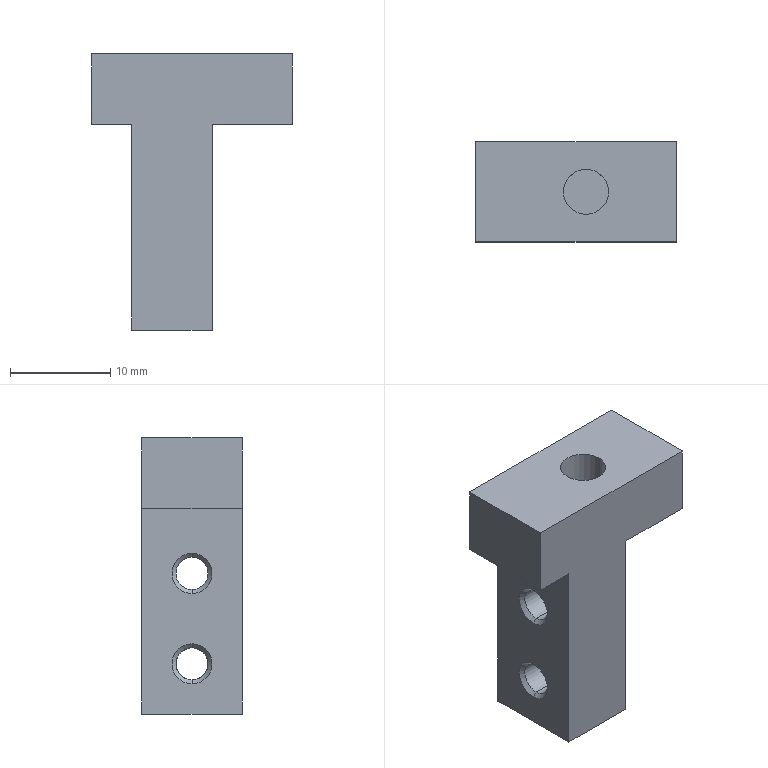Part | SolidWorks | features BaseBody 1 | 1 solid | 25 faces | box 20 x 10 x 27.5 mm | volume 2836 mm3 | plane 11 | cone 8 | cylinder 6 | commonest cylinder face diameters 3.2 x4 4.5 x2
STEP:
#1=CARTESIAN_POINT('',(-16.5,0.,-9.));
#2=VERTEX_POINT('',#1);
#3=CARTESIAN_POINT('',(-12.,0.,-9.));
#4=VERTEX_POINT('',#3);
#5=CARTESIAN_POINT('',(-14.25,0.,-9.));
#6=DIRECTION('',(0.,0.,1.));
#7=DIRECTION('',(1.,0.,0.));
#8=AXIS2_PLACEMENT_3D('',#5,#6,#7);
#9=CIRCLE('',#8,2.25);
#10=EDGE_CURVE('',#2,#4,#9,.T.);
#11=ORIENTED_EDGE('',*,*,#10,.F.);
#12=CARTESIAN_POINT('',(-16.5,0.,-4.5));
#13=VERTEX_POINT('',#12);
#14=CARTESIAN_POINT('',(-16.5,0.,-4.5));
#15=DIRECTION('',(0.,0.,1.));
#16=VECTOR('',#15,1000.);
#17=LINE('',#14,#16);
#18=EDGE_CURVE('',#2,#13,#17,.T.);
#19=ORIENTED_EDGE('',*,*,#18,.T.);
#20=CARTESIAN_POINT('',(-12.,0.,-4.5));
#21=VERTEX_POINT('',#20);
#22=CARTESIAN_POINT('',(-14.25,0.,-4.5));
#23=DIRECTION('',(0.,0.,-1.));
#24=DIRECTION('',(1.,0.,0.));
#25=AXIS2_PLACEMENT_3D('',#22,#23,#24);
#26=CIRCLE('',#25,2.25);
#27=EDGE_CURVE('',#21,#13,#26,.T.);
#28=ORIENTED_EDGE('',*,*,#27,.F.);
#29=CARTESIAN_POINT('',(-12.,0.,-4.5));
#30=DIRECTION('',(0.,0.,1.));
#31=VECTOR('',#30,1000.);
#32=LINE('',#29,#31);
#33=EDGE_CURVE('',#4,#21,#32,.T.);
#34=ORIENTED_EDGE('',*,*,#33,.F.);
#35=EDGE_LOOP('',(#11,#19,#28,#34));
#36=FACE_OUTER_BOUND('',#35,.T.);
#37=CARTESIAN_POINT('',(-14.25,0.,-4.5));
#38=DIRECTION('',(0.,0.,1.));
#39=DIRECTION('',(1.,0.,0.));
#40=AXIS2_PLACEMENT_3D('',#37,#38,#39);
#41=CYLINDRICAL_SURFACE('',#40,2.25);
#42=ADVANCED_FACE('',(#36),#41,.F.);
#43=CARTESIAN_POINT('',(-20.85,0.,-28.6));
#44=VERTEX_POINT('',#43);
#45=CARTESIAN_POINT('',(-20.85,0.,-25.4));
#46=VERTEX_POINT('',#45);
#47=CARTESIAN_POINT('',(-20.85,0.,-27.));
#48=DIRECTION('',(-1.,0.,0.));
#49=DIRECTION('',(0.,0.,-1.));
#50=AXIS2_PLACEMENT_3D('',#47,#48,#49);
#51=CIRCLE('',#50,1.6);
#52=EDGE_CURVE('',#44,#46,#51,.T.);
#53=ORIENTED_EDGE('',*,*,#52,.F.);
#54=CARTESIAN_POINT('',(-21.25,0.,-29.));
#55=VERTEX_POINT('',#54);
#56=CARTESIAN_POINT('',(-21.25,0.,-29.));
#57=DIRECTION('',(-0.7071,0.,-0.7071));
#58=VECTOR('',#57,1000.);
#59=LINE('',#56,#58);
#60=EDGE_CURVE('',#44,#55,#59,.T.);
#61=ORIENTED_EDGE('',*,*,#60,.T.);
#62=CARTESIAN_POINT('',(-21.25,0.,-25.));
#63=VERTEX_POINT('',#62);
#64=CARTESIAN_POINT('',(-21.25,0.,-27.));
#65=DIRECTION('',(1.,0.,0.));
#66=DIRECTION('',(0.,0.,1.));
#67=AXIS2_PLACEMENT_3D('',#64,#65,#66);
#68=CIRCLE('',#67,2.);
#69=EDGE_CURVE('',#63,#55,#68,.T.);
#70=ORIENTED_EDGE('',*,*,#69,.F.);
#71=CARTESIAN_POINT('',(-21.25,0.,-25.));
#72=DIRECTION('',(-0.7071,0.,0.7071));
#73=VECTOR('',#72,1000.);
#74=LINE('',#71,#73);
#75=EDGE_CURVE('',#46,#63,#74,.T.);
#76=ORIENTED_EDGE('',*,*,#75,.F.);
#77=EDGE_LOOP('',(#53,#61,#70,#76));
#78=FACE_OUTER_BOUND('',#77,.T.);
#79=CARTESIAN_POINT('',(-21.25,0.,-27.));
#80=DIRECTION('',(-1.,0.,0.));
#81=DIRECTION('',(0.,0.,1.));
#82=AXIS2_PLACEMENT_3D('',#79,#80,#81);
#83=CONICAL_SURFACE('',#82,2.,0.7854);
#84=ADVANCED_FACE('',(#78),#83,.F.);
#85=CARTESIAN_POINT('',(-20.85,0.,-19.6));
#86=VERTEX_POINT('',#85);
#87=CARTESIAN_POINT('',(-20.85,0.,-16.4));
#88=VERTEX_POINT('',#87);
#89=CARTESIAN_POINT('',(-20.85,0.,-18.));
#90=DIRECTION('',(-1.,0.,0.));
#91=DIRECTION('',(0.,0.,-1.));
#92=AXIS2_PLACEMENT_3D('',#89,#90,#91);
#93=CIRCLE('',#92,1.6);
#94=EDGE_CURVE('',#86,#88,#93,.T.);
#95=ORIENTED_EDGE('',*,*,#94,.F.);
#96=CARTESIAN_POINT('',(-21.25,0.,-20.));
#97=VERTEX_POINT('',#96);
#98=CARTESIAN_POINT('',(-21.25,0.,-20.));
#99=DIRECTION('',(-0.7071,0.,-0.7071));
#100=VECTOR('',#99,1000.);
#101=LINE('',#98,#100);
#102=EDGE_CURVE('',#86,#97,#101,.T.);
#103=ORIENTED_EDGE('',*,*,#102,.T.);
#104=CARTESIAN_POINT('',(-21.25,0.,-16.));
#105=VERTEX_POINT('',#104);
#106=CARTESIAN_POINT('',(-21.25,0.,-18.));
#107=DIRECTION('',(1.,0.,0.));
#108=DIRECTION('',(0.,0.,1.));
#109=AXIS2_PLACEMENT_3D('',#106,#107,#108);
#110=CIRCLE('',#109,2.);
#111=EDGE_CURVE('',#105,#97,#110,.T.);
#112=ORIENTED_EDGE('',*,*,#111,.F.);
#113=CARTESIAN_POINT('',(-21.25,0.,-16.));
#114=DIRECTION('',(-0.7071,0.,0.7071));
#115=VECTOR('',#114,1000.);
#116=LINE('',#113,#115);
#117=EDGE_CURVE('',#88,#105,#116,.T.);
#118=ORIENTED_EDGE('',*,*,#117,.F.);
#119=EDGE_LOOP('',(#95,#103,#112,#118));
#120=FACE_OUTER_BOUND('',#119,.T.);
#121=CARTESIAN_POINT('',(-21.25,0.,-18.));
#122=DIRECTION('',(-1.,0.,0.));
#123=DIRECTION('',(0.,0.,1.));
#124=AXIS2_PLACEMENT_3D('',#121,#122,#123);
#125=CONICAL_SURFACE('',#124,2.,0.7854);
#126=ADVANCED_FACE('',(#120),#125,.F.);
#127=CARTESIAN_POINT('',(-13.65,0.,-16.4));
#128=VERTEX_POINT('',#127);
#129=CARTESIAN_POINT('',(-13.65,0.,-19.6));
#130=VERTEX_POINT('',#129);
#131=CARTESIAN_POINT('',(-13.65,0.,-18.));
#132=DIRECTION('',(1.,0.,0.));
#133=DIRECTION('',(0.,0.,-1.));
#134=AXIS2_PLACEMENT_3D('',#131,#132,#133);
#135=CIRCLE('',#134,1.6);
#136=EDGE_CURVE('',#128,#130,#135,.T.);
#137=ORIENTED_EDGE('',*,*,#136,.F.);
#138=CARTESIAN_POINT('',(-13.25,0.,-16.));
#139=VERTEX_POINT('',#138);
#140=CARTESIAN_POINT('',(-13.25,0.,-16.));
#141=DIRECTION('',(0.7071,0.,0.7071));
#142=VECTOR('',#141,1000.);
#143=LINE('',#140,#142);
#144=EDGE_CURVE('',#128,#139,#143,.T.);
#145=ORIENTED_EDGE('',*,*,#144,.T.);
#146=CARTESIAN_POINT('',(-13.25,0.,-20.));
#147=VERTEX_POINT('',#146);
#148=CARTESIAN_POINT('',(-13.25,0.,-18.));
#149=DIRECTION('',(-1.,0.,0.));
#150=DIRECTION('',(0.,0.,-1.));
#151=AXIS2_PLACEMENT_3D('',#148,#149,#150);
#152=CIRCLE('',#151,2.);
#153=EDGE_CURVE('',#147,#139,#152,.T.);
#154=ORIENTED_EDGE('',*,*,#153,.F.);
#155=CARTESIAN_POINT('',(-13.25,0.,-20.));
#156=DIRECTION('',(0.7071,0.,-0.7071));
#157=VECTOR('',#156,1000.);
#158=LINE('',#155,#157);
#159=EDGE_CURVE('',#130,#147,#158,.T.);
#160=ORIENTED_EDGE('',*,*,#159,.F.);
#161=EDGE_LOOP('',(#137,#145,#154,#160));
#162=FACE_OUTER_BOUND('',#161,.T.);
#163=CARTESIAN_POINT('',(-13.25,0.,-18.));
#164=DIRECTION('',(1.,0.,0.));
#165=DIRECTION('',(0.,0.,-1.));
#166=AXIS2_PLACEMENT_3D('',#163,#164,#165);
#167=CONICAL_SURFACE('',#166,2.,0.7854);
#168=ADVANCED_FACE('',(#162),#167,.F.);
#169=CARTESIAN_POINT('',(-13.65,-1.6,-27.));
#170=VERTEX_POINT('',#169);
#171=CARTESIAN_POINT('',(-13.65,0.,-28.6));
#172=VERTEX_POINT('',#171);
#173=CARTESIAN_POINT('',(-13.65,0.,-27.));
#174=DIRECTION('',(1.,0.,0.));
#175=DIRECTION('',(0.,0.,-1.));
#176=AXIS2_PLACEMENT_3D('',#173,#174,#175);
#177=CIRCLE('',#176,1.6);
#178=EDGE_CURVE('',#170,#172,#177,.T.);
#179=ORIENTED_EDGE('',*,*,#178,.F.);
#180=CARTESIAN_POINT('',(-13.25,-2.,-27.));
#181=VERTEX_POINT('',#180);
#182=CARTESIAN_POINT('',(-13.25,-2.,-27.));
#183=DIRECTION('',(0.7071,-0.7071,0.));
#184=VECTOR('',#183,1000.);
#185=LINE('',#182,#184);
#186=EDGE_CURVE('',#170,#181,#185,.T.);
#187=ORIENTED_EDGE('',*,*,#186,.T.);
#188=CARTESIAN_POINT('',(-13.25,2.,-27.));
#189=VERTEX_POINT('',#188);
#190=CARTESIAN_POINT('',(-13.25,0.,-27.));
#191=DIRECTION('',(-1.,0.,0.));
#192=DIRECTION('',(0.,1.,0.));
#193=AXIS2_PLACEMENT_3D('',#190,#191,#192);
#194=CIRCLE('',#193,2.);
#195=EDGE_CURVE('',#189,#181,#194,.T.);
#196=ORIENTED_EDGE('',*,*,#195,.F.);
#197=CARTESIAN_POINT('',(-13.65,1.6,-27.));
#198=VERTEX_POINT('',#197);
#199=CARTESIAN_POINT('',(-13.25,2.,-27.));
#200=DIRECTION('',(0.7071,0.7071,0.));
#201=VECTOR('',#200,1000.);
#202=LINE('',#199,#201);
#203=EDGE_CURVE('',#198,#189,#202,.T.);
#204=ORIENTED_EDGE('',*,*,#203,.F.);
#205=CARTESIAN_POINT('',(-13.65,0.,-27.));
#206=DIRECTION('',(1.,0.,0.));
#207=DIRECTION('',(0.,0.,-1.));
#208=AXIS2_PLACEMENT_3D('',#205,#206,#207);
#209=CIRCLE('',#208,1.6);
#210=EDGE_CURVE('',#172,#198,#209,.T.);
#211=ORIENTED_EDGE('',*,*,#210,.F.);
#212=EDGE_LOOP('',(#179,#187,#196,#204,#211));
#213=FACE_OUTER_BOUND('',#212,.T.);
#214=CARTESIAN_POINT('',(-13.25,0.,-27.));
#215=DIRECTION('',(1.,0.,0.));
#216=DIRECTION('',(0.,1.,0.));
#217=AXIS2_PLACEMENT_3D('',#214,#215,#216);
#218=CONICAL_SURFACE('',#217,2.,0.7854);
#219=ADVANCED_FACE('',(#213),#218,.F.);
#220=ORIENTED_EDGE('',*,*,#52,.T.);
#221=CARTESIAN_POINT('',(-13.65,0.,-25.4));
#222=VERTEX_POINT('',#221);
#223=CARTESIAN_POINT('',(21.25,0.,-25.4));
#224=DIRECTION('',(1.,0.,0.));
#225=VECTOR('',#224,1000.);
#226=LINE('',#223,#225);
#227=EDGE_CURVE('',#46,#222,#226,.T.);
#228=ORIENTED_EDGE('',*,*,#227,.T.);
#229=CARTESIAN_POINT('',(-13.65,0.,-27.));
#230=DIRECTION('',(1.,0.,0.));
#231=DIRECTION('',(0.,0.,-1.));
#232=AXIS2_PLACEMENT_3D('',#229,#230,#231);
#233=CIRCLE('',#232,1.6);
#234=EDGE_CURVE('',#222,#170,#233,.T.);
#235=ORIENTED_EDGE('',*,*,#234,.T.);
#236=ORIENTED_EDGE('',*,*,#178,.T.);
#237=CARTESIAN_POINT('',(21.25,0.,-28.6));
#238=DIRECTION('',(1.,0.,0.));
#239=VECTOR('',#238,1000.);
#240=LINE('',#237,#239);
#241=EDGE_CURVE('',#44,#172,#240,.T.);
#242=ORIENTED_EDGE('',*,*,#241,.F.);
#243=EDGE_LOOP('',(#220,#228,#235,#236,#242));
#244=FACE_OUTER_BOUND('',#243,.T.);
#245=CARTESIAN_POINT('',(21.25,0.,-27.));
#246=DIRECTION('',(1.,0.,0.));
#247=DIRECTION('',(0.,0.,-1.));
#248=AXIS2_PLACEMENT_3D('',#245,#246,#247);
#249=CYLINDRICAL_SURFACE('',#248,1.6);
#250=ADVANCED_FACE('',(#244),#249,.F.);
#251=ORIENTED_EDGE('',*,*,#94,.T.);
#252=CARTESIAN_POINT('',(21.25,0.,-16.4));
#253=DIRECTION('',(1.,0.,0.));
#254=VECTOR('',#253,1000.);
#255=LINE('',#252,#254);
#256=EDGE_CURVE('',#88,#128,#255,.T.);
#257=ORIENTED_EDGE('',*,*,#256,.T.);
#258=ORIENTED_EDGE('',*,*,#136,.T.);
#259=CARTESIAN_POINT('',(21.25,0.,-19.6));
#260=DIRECTION('',(1.,0.,0.));
#261=VECTOR('',#260,1000.);
#262=LINE('',#259,#261);
#263=EDGE_CURVE('',#86,#130,#262,.T.);
#264=ORIENTED_EDGE('',*,*,#263,.F.);
#265=EDGE_LOOP('',(#251,#257,#258,#264));
#266=FACE_OUTER_BOUND('',#265,.T.);
#267=CARTESIAN_POINT('',(21.25,0.,-18.));
#268=DIRECTION('',(1.,0.,0.));
#269=DIRECTION('',(0.,0.,-1.));
#270=AXIS2_PLACEMENT_3D('',#267,#268,#269);
#271=CYLINDRICAL_SURFACE('',#270,1.6);
#272=ADVANCED_FACE('',(#266),#271,.F.);
#273=CARTESIAN_POINT('',(-25.25,5.,-4.5));
#274=VERTEX_POINT('',#273);
#275=CARTESIAN_POINT('',(-5.25,5.,-4.5));
#276=VERTEX_POINT('',#275);
#277=CARTESIAN_POINT('',(0.,5.,-4.5));
#278=DIRECTION('',(1.,0.,0.));
#279=VECTOR('',#278,1000.);
#280=LINE('',#277,#279);
#281=EDGE_CURVE('',#274,#276,#280,.T.);
#282=ORIENTED_EDGE('',*,*,#281,.T.);
#283=CARTESIAN_POINT('',(-5.25,5.,-11.5));
#284=VERTEX_POINT('',#283);
#285=CARTESIAN_POINT('',(-5.25,5.,0.));
#286=DIRECTION('',(0.,0.,-1.));
#287=VECTOR('',#286,1000.);
#288=LINE('',#285,#287);
#289=EDGE_CURVE('',#276,#284,#288,.T.);
#290=ORIENTED_EDGE('',*,*,#289,.T.);
#291=CARTESIAN_POINT('',(-13.25,5.,-11.5));
#292=VERTEX_POINT('',#291);
#293=CARTESIAN_POINT('',(0.,5.,-11.5));
#294=DIRECTION('',(-1.,0.,0.));
#295=VECTOR('',#294,1000.);
#296=LINE('',#293,#295);
#297=EDGE_CURVE('',#284,#292,#296,.T.);
#298=ORIENTED_EDGE('',*,*,#297,.T.);
#299=CARTESIAN_POINT('',(-13.25,5.,-32.));
#300=VERTEX_POINT('',#299);
#301=CARTESIAN_POINT('',(-13.25,5.,0.));
#302=DIRECTION('',(0.,0.,-1.));
#303=VECTOR('',#302,1000.);
#304=LINE('',#301,#303);
#305=EDGE_CURVE('',#292,#300,#304,.T.);
#306=ORIENTED_EDGE('',*,*,#305,.T.);
#307=CARTESIAN_POINT('',(-21.25,5.,-32.));
#308=VERTEX_POINT('',#307);
#309=CARTESIAN_POINT('',(0.,5.,-32.));
#310=DIRECTION('',(-1.,0.,0.));
#311=VECTOR('',#310,1000.);
#312=LINE('',#309,#311);
#313=EDGE_CURVE('',#300,#308,#312,.T.);
#314=ORIENTED_EDGE('',*,*,#313,.T.);
#315=CARTESIAN_POINT('',(-21.25,5.,-11.5));
#316=VERTEX_POINT('',#315);
#317=CARTESIAN_POINT('',(-21.25,5.,0.));
#318=DIRECTION('',(0.,0.,1.));
#319=VECTOR('',#318,1000.);
#320=LINE('',#317,#319);
#321=EDGE_CURVE('',#308,#316,#320,.T.);
#322=ORIENTED_EDGE('',*,*,#321,.T.);
#323=CARTESIAN_POINT('',(-25.25,5.,-11.5));
#324=VERTEX_POINT('',#323);
#325=CARTESIAN_POINT('',(0.,5.,-11.5));
#326=DIRECTION('',(-1.,0.,0.));
#327=VECTOR('',#326,1000.);
#328=LINE('',#325,#327);
#329=EDGE_CURVE('',#316,#324,#328,.T.);
#330=ORIENTED_EDGE('',*,*,#329,.T.);
#331=CARTESIAN_POINT('',(-25.25,5.,0.));
#332=DIRECTION('',(0.,0.,1.));
#333=VECTOR('',#332,1000.);
#334=LINE('',#331,#333);
#335=EDGE_CURVE('',#324,#274,#334,.T.);
#336=ORIENTED_EDGE('',*,*,#335,.T.);
#337=EDGE_LOOP('',(#282,#290,#298,#306,#314,#322,#330,#336));
#338=FACE_OUTER_BOUND('',#337,.T.);
#339=CARTESIAN_POINT('',(0.,5.,0.));
#340=DIRECTION('',(0.,1.,0.));
#341=DIRECTION('',(0.,0.,1.));
#342=AXIS2_PLACEMENT_3D('',#339,#340,#341);
#343=PLANE('',#342);
#344=ADVANCED_FACE('',(#338),#343,.T.);
#345=CARTESIAN_POINT('',(-5.25,-5.,-4.5));
#346=VERTEX_POINT('',#345);
#347=CARTESIAN_POINT('',(-5.25,-5.,-11.5));
#348=VERTEX_POINT('',#347);
#349=CARTESIAN_POINT('',(-5.25,-5.,-4.5));
#350=DIRECTION('',(0.,0.,-1.));
#351=VECTOR('',#350,1000.);
#352=LINE('',#349,#351);
#353=EDGE_CURVE('',#346,#348,#352,.T.);
#354=ORIENTED_EDGE('',*,*,#353,.T.);
#355=CARTESIAN_POINT('',(-5.25,-5.,-11.5));
#356=DIRECTION('',(0.,1.,0.));
#357=VECTOR('',#356,1000.);
#358=LINE('',#355,#357);
#359=EDGE_CURVE('',#348,#284,#358,.T.);
#360=ORIENTED_EDGE('',*,*,#359,.T.);
#361=ORIENTED_EDGE('',*,*,#289,.F.);
#362=CARTESIAN_POINT('',(-5.25,-5.,-4.5));
#363=DIRECTION('',(0.,-1.,0.));
#364=VECTOR('',#363,1000.);
#365=LINE('',#362,#364);
#366=EDGE_CURVE('',#276,#346,#365,.T.);
#367=ORIENTED_EDGE('',*,*,#366,.T.);
#368=EDGE_LOOP('',(#354,#360,#361,#367));
#369=FACE_OUTER_BOUND('',#368,.T.);
#370=CARTESIAN_POINT('',(-5.25,-5.,-4.5));
#371=DIRECTION('',(1.,0.,0.));
#372=DIRECTION('',(0.,0.,-1.));
#373=AXIS2_PLACEMENT_3D('',#370,#371,#372);
#374=PLANE('',#373);
#375=ADVANCED_FACE('',(#369),#374,.T.);
#376=ORIENTED_EDGE('',*,*,#27,.T.);
#377=CARTESIAN_POINT('',(-14.25,0.,-4.5));
#378=DIRECTION('',(0.,0.,-1.));
#379=DIRECTION('',(1.,0.,0.));
#380=AXIS2_PLACEMENT_3D('',#377,#378,#379);
#381=CIRCLE('',#380,2.25);
#382=EDGE_CURVE('',#13,#21,#381,.T.);
#383=ORIENTED_EDGE('',*,*,#382,.T.);
#384=EDGE_LOOP('',(#376,#383));
#385=FACE_BOUND('',#384,.T.);
#386=CARTESIAN_POINT('',(-25.25,-5.,-4.5));
#387=VERTEX_POINT('',#386);
#388=CARTESIAN_POINT('',(-25.25,-5.,-4.5));
#389=DIRECTION('',(1.,0.,0.));
#390=VECTOR('',#389,1000.);
#391=LINE('',#388,#390);
#392=EDGE_CURVE('',#387,#346,#391,.T.);
#393=ORIENTED_EDGE('',*,*,#392,.T.);
#394=ORIENTED_EDGE('',*,*,#366,.F.);
#395=ORIENTED_EDGE('',*,*,#281,.F.);
#396=CARTESIAN_POINT('',(-25.25,-5.,-4.5));
#397=DIRECTION('',(0.,-1.,0.));
#398=VECTOR('',#397,1000.);
#399=LINE('',#396,#398);
#400=EDGE_CURVE('',#274,#387,#399,.T.);
#401=ORIENTED_EDGE('',*,*,#400,.T.);
#402=EDGE_LOOP('',(#393,#394,#395,#401));
#403=FACE_OUTER_BOUND('',#402,.T.);
#404=CARTESIAN_POINT('',(-25.25,-5.,-4.5));
#405=DIRECTION('',(0.,0.,1.));
#406=DIRECTION('',(1.,0.,0.));
#407=AXIS2_PLACEMENT_3D('',#404,#405,#406);
#408=PLANE('',#407);
#409=ADVANCED_FACE('',(#385,#403),#408,.T.);
#410=CARTESIAN_POINT('',(-25.25,-5.,-11.5));
#411=VERTEX_POINT('',#410);
#412=CARTESIAN_POINT('',(-25.25,-5.,-11.5));
#413=DIRECTION('',(0.,0.,1.));
#414=VECTOR('',#413,1000.);
#415=LINE('',#412,#414);
#416=EDGE_CURVE('',#411,#387,#415,.T.);
#417=ORIENTED_EDGE('',*,*,#416,.T.);
#418=ORIENTED_EDGE('',*,*,#400,.F.);
#419=ORIENTED_EDGE('',*,*,#335,.F.);
#420=CARTESIAN_POINT('',(-25.25,-5.,-11.5));
#421=DIRECTION('',(0.,-1.,0.));
#422=VECTOR('',#421,1000.);
#423=LINE('',#420,#422);
#424=EDGE_CURVE('',#324,#411,#423,.T.);
#425=ORIENTED_EDGE('',*,*,#424,.T.);
#426=EDGE_LOOP('',(#417,#418,#419,#425));
#427=FACE_OUTER_BOUND('',#426,.T.);
#428=CARTESIAN_POINT('',(-25.25,-5.,-11.5));
#429=DIRECTION('',(-1.,0.,0.));
#430=DIRECTION('',(0.,0.,1.));
#431=AXIS2_PLACEMENT_3D('',#428,#429,#430);
#432=PLANE('',#431);
#433=ADVANCED_FACE('',(#427),#432,.T.);
#434=CARTESIAN_POINT('',(-21.25,-5.,-11.5));
#435=VERTEX_POINT('',#434);
#436=CARTESIAN_POINT('',(-21.25,-5.,-11.5));
#437=DIRECTION('',(-1.,0.,0.));
#438=VECTOR('',#437,1000.);
#439=LINE('',#436,#438);
#440=EDGE_CURVE('',#435,#411,#439,.T.);
#441=ORIENTED_EDGE('',*,*,#440,.T.);
#442=ORIENTED_EDGE('',*,*,#424,.F.);
#443=ORIENTED_EDGE('',*,*,#329,.F.);
#444=CARTESIAN_POINT('',(-21.25,-5.,-11.5));
#445=DIRECTION('',(0.,-1.,0.));
#446=VECTOR('',#445,1000.);
#447=LINE('',#444,#446);
#448=EDGE_CURVE('',#316,#435,#447,.T.);
#449=ORIENTED_EDGE('',*,*,#448,.T.);
#450=EDGE_LOOP('',(#441,#442,#443,#449));
#451=FACE_OUTER_BOUND('',#450,.T.);
#452=CARTESIAN_POINT('',(-21.25,-5.,-11.5));
#453=DIRECTION('',(0.,0.,-1.));
#454=DIRECTION('',(-1.,0.,0.));
#455=AXIS2_PLACEMENT_3D('',#452,#453,#454);
#456=PLANE('',#455);
#457=ADVANCED_FACE('',(#451),#456,.T.);
#458=ORIENTED_EDGE('',*,*,#69,.T.);
#459=CARTESIAN_POINT('',(-21.25,0.,-27.));
#460=DIRECTION('',(1.,0.,0.));
#461=DIRECTION('',(0.,0.,1.));
#462=AXIS2_PLACEMENT_3D('',#459,#460,#461);
#463=CIRCLE('',#462,2.);
#464=EDGE_CURVE('',#55,#63,#463,.T.);
#465=ORIENTED_EDGE('',*,*,#464,.T.);
#466=EDGE_LOOP('',(#458,#465));
#467=FACE_BOUND('',#466,.T.);
#468=ORIENTED_EDGE('',*,*,#111,.T.);
#469=CARTESIAN_POINT('',(-21.25,0.,-18.));
#470=DIRECTION('',(1.,0.,0.));
#471=DIRECTION('',(0.,0.,1.));
#472=AXIS2_PLACEMENT_3D('',#469,#470,#471);
#473=CIRCLE('',#472,2.);
#474=EDGE_CURVE('',#97,#105,#473,.T.);
#475=ORIENTED_EDGE('',*,*,#474,.T.);
#476=EDGE_LOOP('',(#468,#475));
#477=FACE_BOUND('',#476,.T.);
#478=CARTESIAN_POINT('',(-21.25,-5.,-32.));
#479=VERTEX_POINT('',#478);
#480=CARTESIAN_POINT('',(-21.25,-5.,-32.));
#481=DIRECTION('',(0.,0.,1.));
#482=VECTOR('',#481,1000.);
#483=LINE('',#480,#482);
#484=EDGE_CURVE('',#479,#435,#483,.T.);
#485=ORIENTED_EDGE('',*,*,#484,.T.);
#486=ORIENTED_EDGE('',*,*,#448,.F.);
#487=ORIENTED_EDGE('',*,*,#321,.F.);
#488=CARTESIAN_POINT('',(-21.25,-5.,-32.));
#489=DIRECTION('',(0.,-1.,0.));
#490=VECTOR('',#489,1000.);
#491=LINE('',#488,#490);
#492=EDGE_CURVE('',#308,#479,#491,.T.);
#493=ORIENTED_EDGE('',*,*,#492,.T.);
#494=EDGE_LOOP('',(#485,#486,#487,#493));
#495=FACE_OUTER_BOUND('',#494,.T.);
#496=CARTESIAN_POINT('',(-21.25,-5.,-32.));
#497=DIRECTION('',(-1.,0.,0.));
#498=DIRECTION('',(0.,0.,1.));
#499=AXIS2_PLACEMENT_3D('',#496,#497,#498);
#500=PLANE('',#499);
#501=ADVANCED_FACE('',(#467,#477,#495),#500,.T.);
#502=CARTESIAN_POINT('',(-13.25,-5.,-32.));
#503=VERTEX_POINT('',#502);
#504=CARTESIAN_POINT('',(-13.25,-5.,-32.));
#505=DIRECTION('',(-1.,0.,0.));
#506=VECTOR('',#505,1000.);
#507=LINE('',#504,#506);
#508=EDGE_CURVE('',#503,#479,#507,.T.);
#509=ORIENTED_EDGE('',*,*,#508,.T.);
#510=ORIENTED_EDGE('',*,*,#492,.F.);
#511=ORIENTED_EDGE('',*,*,#313,.F.);
#512=CARTESIAN_POINT('',(-13.25,-5.,-32.));
#513=DIRECTION('',(0.,-1.,0.));
#514=VECTOR('',#513,1000.);
#515=LINE('',#512,#514);
#516=EDGE_CURVE('',#300,#503,#515,.T.);
#517=ORIENTED_EDGE('',*,*,#516,.T.);
#518=EDGE_LOOP('',(#509,#510,#511,#517));
#519=FACE_OUTER_BOUND('',#518,.T.);
#520=CARTESIAN_POINT('',(-13.25,-5.,-32.));
#521=DIRECTION('',(0.,0.,-1.));
#522=DIRECTION('',(-1.,0.,0.));
#523=AXIS2_PLACEMENT_3D('',#520,#521,#522);
#524=PLANE('',#523);
#525=ADVANCED_FACE('',(#519),#524,.T.);
#526=ORIENTED_EDGE('',*,*,#153,.T.);
#527=CARTESIAN_POINT('',(-13.25,0.,-18.));
#528=DIRECTION('',(-1.,0.,0.));
#529=DIRECTION('',(0.,0.,-1.));
#530=AXIS2_PLACEMENT_3D('',#527,#528,#529);
#531=CIRCLE('',#530,2.);
#532=EDGE_CURVE('',#139,#147,#531,.T.);
#533=ORIENTED_EDGE('',*,*,#532,.T.);
#534=EDGE_LOOP('',(#526,#533));
#535=FACE_BOUND('',#534,.T.);
#536=ORIENTED_EDGE('',*,*,#195,.T.);
#537=CARTESIAN_POINT('',(-13.25,0.,-27.));
#538=DIRECTION('',(-1.,0.,0.));
#539=DIRECTION('',(0.,1.,0.));
#540=AXIS2_PLACEMENT_3D('',#537,#538,#539);
#541=CIRCLE('',#540,2.);
#542=EDGE_CURVE('',#181,#189,#541,.T.);
#543=ORIENTED_EDGE('',*,*,#542,.T.);
#544=EDGE_LOOP('',(#536,#543));
#545=FACE_BOUND('',#544,.T.);
#546=CARTESIAN_POINT('',(-13.25,-5.,-11.5));
#547=VERTEX_POINT('',#546);
#548=CARTESIAN_POINT('',(-13.25,-5.,-11.5));
#549=DIRECTION('',(0.,0.,-1.));
#550=VECTOR('',#549,1000.);
#551=LINE('',#548,#550);
#552=EDGE_CURVE('',#547,#503,#551,.T.);
#553=ORIENTED_EDGE('',*,*,#552,.T.);
#554=ORIENTED_EDGE('',*,*,#516,.F.);
#555=ORIENTED_EDGE('',*,*,#305,.F.);
#556=CARTESIAN_POINT('',(-13.25,-5.,-11.5));
#557=DIRECTION('',(0.,-1.,0.));
#558=VECTOR('',#557,1000.);
#559=LINE('',#556,#558);
#560=EDGE_CURVE('',#292,#547,#559,.T.);
#561=ORIENTED_EDGE('',*,*,#560,.T.);
#562=EDGE_LOOP('',(#553,#554,#555,#561));
#563=FACE_OUTER_BOUND('',#562,.T.);
#564=CARTESIAN_POINT('',(-13.25,-5.,-11.5));
#565=DIRECTION('',(1.,0.,0.));
#566=DIRECTION('',(0.,0.,-1.));
#567=AXIS2_PLACEMENT_3D('',#564,#565,#566);
#568=PLANE('',#567);
#569=ADVANCED_FACE('',(#535,#545,#563),#568,.T.);
#570=CARTESIAN_POINT('',(-5.25,-5.,-11.5));
#571=DIRECTION('',(-1.,0.,0.));
#572=VECTOR('',#571,1000.);
#573=LINE('',#570,#572);
#574=EDGE_CURVE('',#348,#547,#573,.T.);
#575=ORIENTED_EDGE('',*,*,#574,.T.);
#576=ORIENTED_EDGE('',*,*,#560,.F.);
#577=ORIENTED_EDGE('',*,*,#297,.F.);
#578=ORIENTED_EDGE('',*,*,#359,.F.);
#579=EDGE_LOOP('',(#575,#576,#577,#578));
#580=FACE_OUTER_BOUND('',#579,.T.);
#581=CARTESIAN_POINT('',(-5.25,-5.,-11.5));
#582=DIRECTION('',(0.,0.,-1.));
#583=DIRECTION('',(-1.,0.,0.));
#584=AXIS2_PLACEMENT_3D('',#581,#582,#583);
#585=PLANE('',#584);
#586=ADVANCED_FACE('',(#580),#585,.T.);
#587=ORIENTED_EDGE('',*,*,#484,.F.);
#588=ORIENTED_EDGE('',*,*,#508,.F.);
#589=ORIENTED_EDGE('',*,*,#552,.F.);
#590=ORIENTED_EDGE('',*,*,#574,.F.);
#591=ORIENTED_EDGE('',*,*,#353,.F.);
#592=ORIENTED_EDGE('',*,*,#392,.F.);
#593=ORIENTED_EDGE('',*,*,#416,.F.);
#594=ORIENTED_EDGE('',*,*,#440,.F.);
#595=EDGE_LOOP('',(#587,#588,#589,#590,#591,#592,#593,#594));
#596=FACE_OUTER_BOUND('',#595,.T.);
#597=CARTESIAN_POINT('',(0.,-5.,0.));
#598=DIRECTION('',(0.,1.,0.));
#599=DIRECTION('',(0.,0.,1.));
#600=AXIS2_PLACEMENT_3D('',#597,#598,#599);
#601=PLANE('',#600);
#602=ADVANCED_FACE('',(#596),#601,.F.);
#603=ORIENTED_EDGE('',*,*,#18,.F.);
#604=CARTESIAN_POINT('',(-14.25,0.,-9.));
#605=DIRECTION('',(0.,0.,1.));
#606=DIRECTION('',(1.,0.,0.));
#607=AXIS2_PLACEMENT_3D('',#604,#605,#606);
#608=CIRCLE('',#607,2.25);
#609=EDGE_CURVE('',#4,#2,#608,.T.);
#610=ORIENTED_EDGE('',*,*,#609,.F.);
#611=ORIENTED_EDGE('',*,*,#33,.T.);
#612=ORIENTED_EDGE('',*,*,#382,.F.);
#613=EDGE_LOOP('',(#603,#610,#611,#612));
#614=FACE_OUTER_BOUND('',#613,.T.);
#615=CARTESIAN_POINT('',(-14.25,0.,-4.5));
#616=DIRECTION('',(0.,0.,1.));
#617=DIRECTION('',(1.,0.,0.));
#618=AXIS2_PLACEMENT_3D('',#615,#616,#617);
#619=CYLINDRICAL_SURFACE('',#618,2.25);
#620=ADVANCED_FACE('',(#614),#619,.F.);
#621=ORIENTED_EDGE('',*,*,#60,.F.);
#622=CARTESIAN_POINT('',(-20.85,0.,-27.));
#623=DIRECTION('',(-1.,0.,0.));
#624=DIRECTION('',(0.,0.,-1.));
#625=AXIS2_PLACEMENT_3D('',#622,#623,#624);
#626=CIRCLE('',#625,1.6);
#627=EDGE_CURVE('',#46,#44,#626,.T.);
#628=ORIENTED_EDGE('',*,*,#627,.F.);
#629=ORIENTED_EDGE('',*,*,#75,.T.);
#630=ORIENTED_EDGE('',*,*,#464,.F.);
#631=EDGE_LOOP('',(#621,#628,#629,#630));
#632=FACE_OUTER_BOUND('',#631,.T.);
#633=CARTESIAN_POINT('',(-21.25,0.,-27.));
#634=DIRECTION('',(-1.,0.,0.));
#635=DIRECTION('',(0.,0.,1.));
#636=AXIS2_PLACEMENT_3D('',#633,#634,#635);
#637=CONICAL_SURFACE('',#636,2.,0.7854);
#638=ADVANCED_FACE('',(#632),#637,.F.);
#639=ORIENTED_EDGE('',*,*,#102,.F.);
#640=CARTESIAN_POINT('',(-20.85,0.,-18.));
#641=DIRECTION('',(-1.,0.,0.));
#642=DIRECTION('',(0.,0.,-1.));
#643=AXIS2_PLACEMENT_3D('',#640,#641,#642);
#644=CIRCLE('',#643,1.6);
#645=EDGE_CURVE('',#88,#86,#644,.T.);
#646=ORIENTED_EDGE('',*,*,#645,.F.);
#647=ORIENTED_EDGE('',*,*,#117,.T.);
#648=ORIENTED_EDGE('',*,*,#474,.F.);
#649=EDGE_LOOP('',(#639,#646,#647,#648));
#650=FACE_OUTER_BOUND('',#649,.T.);
#651=CARTESIAN_POINT('',(-21.25,0.,-18.));
#652=DIRECTION('',(-1.,0.,0.));
#653=DIRECTION('',(0.,0.,1.));
#654=AXIS2_PLACEMENT_3D('',#651,#652,#653);
#655=CONICAL_SURFACE('',#654,2.,0.7854);
#656=ADVANCED_FACE('',(#650),#655,.F.);
#657=ORIENTED_EDGE('',*,*,#144,.F.);
#658=CARTESIAN_POINT('',(-13.65,0.,-18.));
#659=DIRECTION('',(1.,0.,0.));
#660=DIRECTION('',(0.,0.,-1.));
#661=AXIS2_PLACEMENT_3D('',#658,#659,#660);
#662=CIRCLE('',#661,1.6);
#663=EDGE_CURVE('',#130,#128,#662,.T.);
#664=ORIENTED_EDGE('',*,*,#663,.F.);
#665=ORIENTED_EDGE('',*,*,#159,.T.);
#666=ORIENTED_EDGE('',*,*,#532,.F.);
#667=EDGE_LOOP('',(#657,#664,#665,#666));
#668=FACE_OUTER_BOUND('',#667,.T.);
#669=CARTESIAN_POINT('',(-13.25,0.,-18.));
#670=DIRECTION('',(1.,0.,0.));
#671=DIRECTION('',(0.,0.,-1.));
#672=AXIS2_PLACEMENT_3D('',#669,#670,#671);
#673=CONICAL_SURFACE('',#672,2.,0.7854);
#674=ADVANCED_FACE('',(#668),#673,.F.);
#675=ORIENTED_EDGE('',*,*,#186,.F.);
#676=ORIENTED_EDGE('',*,*,#234,.F.);
#677=CARTESIAN_POINT('',(-13.65,0.,-27.));
#678=DIRECTION('',(1.,0.,0.));
#679=DIRECTION('',(0.,0.,-1.));
#680=AXIS2_PLACEMENT_3D('',#677,#678,#679);
#681=CIRCLE('',#680,1.6);
#682=EDGE_CURVE('',#198,#222,#681,.T.);
#683=ORIENTED_EDGE('',*,*,#682,.F.);
#684=ORIENTED_EDGE('',*,*,#203,.T.);
#685=ORIENTED_EDGE('',*,*,#542,.F.);
#686=EDGE_LOOP('',(#675,#676,#683,#684,#685));
#687=FACE_OUTER_BOUND('',#686,.T.);
#688=CARTESIAN_POINT('',(-13.25,0.,-27.));
#689=DIRECTION('',(1.,0.,0.));
#690=DIRECTION('',(0.,1.,0.));
#691=AXIS2_PLACEMENT_3D('',#688,#689,#690);
#692=CONICAL_SURFACE('',#691,2.,0.7854);
#693=ADVANCED_FACE('',(#687),#692,.F.);
#694=ORIENTED_EDGE('',*,*,#609,.T.);
#695=ORIENTED_EDGE('',*,*,#10,.T.);
#696=EDGE_LOOP('',(#694,#695));
#697=FACE_OUTER_BOUND('',#696,.T.);
#698=CARTESIAN_POINT('',(0.,-5.,-9.));
#699=DIRECTION('',(0.,0.,1.));
#700=DIRECTION('',(1.,0.,0.));
#701=AXIS2_PLACEMENT_3D('',#698,#699,#700);
#702=PLANE('',#701);
#703=ADVANCED_FACE('',(#697),#702,.T.);
#704=ORIENTED_EDGE('',*,*,#227,.F.);
#705=ORIENTED_EDGE('',*,*,#627,.T.);
#706=ORIENTED_EDGE('',*,*,#241,.T.);
#707=ORIENTED_EDGE('',*,*,#210,.T.);
#708=ORIENTED_EDGE('',*,*,#682,.T.);
#709=EDGE_LOOP('',(#704,#705,#706,#707,#708));
#710=FACE_OUTER_BOUND('',#709,.T.);
#711=CARTESIAN_POINT('',(21.25,0.,-27.));
#712=DIRECTION('',(1.,0.,0.));
#713=DIRECTION('',(0.,0.,-1.));
#714=AXIS2_PLACEMENT_3D('',#711,#712,#713);
#715=CYLINDRICAL_SURFACE('',#714,1.6);
#716=ADVANCED_FACE('',(#710),#715,.F.);
#717=ORIENTED_EDGE('',*,*,#256,.F.);
#718=ORIENTED_EDGE('',*,*,#645,.T.);
#719=ORIENTED_EDGE('',*,*,#263,.T.);
#720=ORIENTED_EDGE('',*,*,#663,.T.);
#721=EDGE_LOOP('',(#717,#718,#719,#720));
#722=FACE_OUTER_BOUND('',#721,.T.);
#723=CARTESIAN_POINT('',(21.25,0.,-18.));
#724=DIRECTION('',(1.,0.,0.));
#725=DIRECTION('',(0.,0.,-1.));
#726=AXIS2_PLACEMENT_3D('',#723,#724,#725);
#727=CYLINDRICAL_SURFACE('',#726,1.6);
#728=ADVANCED_FACE('',(#722),#727,.F.);
#729=CLOSED_SHELL('',(#42,#84,#126,#168,#219,#250,#272,#344,#375,#409,#433,#457,#501,#525,#569,#586,#602,#620,#638,#656,#674,#693,#703,#716,#728));
#730=MANIFOLD_SOLID_BREP('',#729);
#731=CARTESIAN_POINT('',(0.,0.,0.));
#732=DIRECTION('',(0.,0.,1.));
#733=DIRECTION('',(1.,0.,0.));
#734=AXIS2_PLACEMENT_3D('',#731,#732,#733);
#735=(LENGTH_UNIT()NAMED_UNIT(*)SI_UNIT(.MILLI.,.METRE.));
#736=UNCERTAINTY_MEASURE_WITH_UNIT(LENGTH_MEASURE(0.00001),#735,'','');
#737=(NAMED_UNIT(*)PLANE_ANGLE_UNIT()SI_UNIT($,.RADIAN.));
#738=(NAMED_UNIT(*)SI_UNIT($,.STERADIAN.)SOLID_ANGLE_UNIT());
#739=(GEOMETRIC_REPRESENTATION_CONTEXT(3)GLOBAL_UNCERTAINTY_ASSIGNED_CONTEXT((#736))GLOBAL_UNIT_ASSIGNED_CONTEXT((#735,#737,#738))REPRESENTATION_CONTEXT('',''));
#740=ADVANCED_BREP_SHAPE_REPRESENTATION('',(#730,#734),#739);